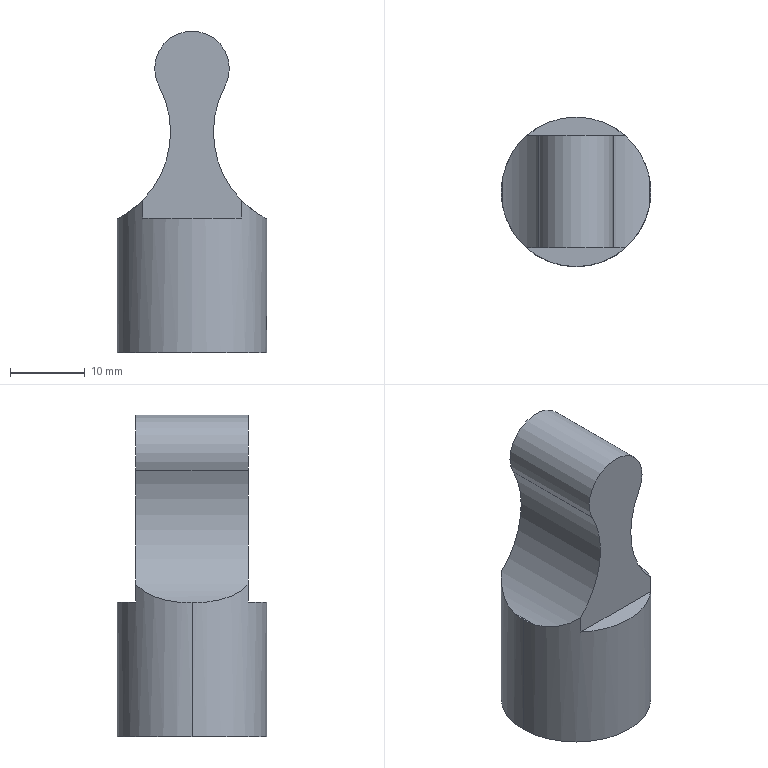Part | STEP file | Seal sleeve 5 | 1 solid | 17 faces | box 20 x 20 x 43 mm | volume 8055 mm3 | cylinder 9 | plane 8 | commonest cylinder face diameters 10 x3 2.5 x2 20 x2 26 x2